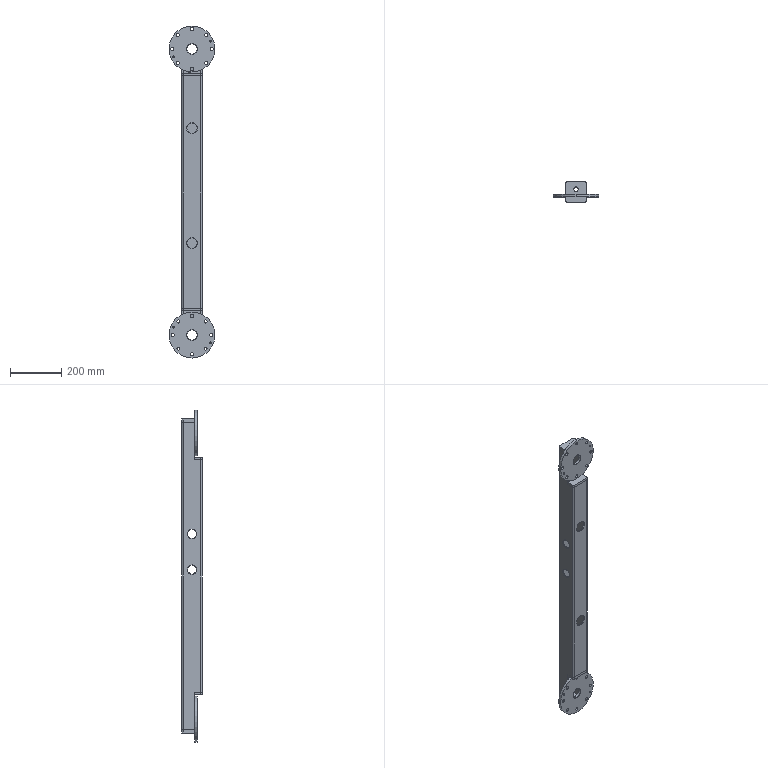Part | SolidWorks | features ICE 8, HoleWzd 6, Chamfer 4, Cut 2, Extrusion 1, Fillet 1, MoveCopyBody 1 | 7 solids | 158 faces | box 180 x 80 x 1300 mm | volume 2167935 mm3 | cylinder 86 | plane 44 | cone 28 | commonest cylinder face diameters 12 x32 10 x12 40 x12 6 x8 35 x8 6.8 x6